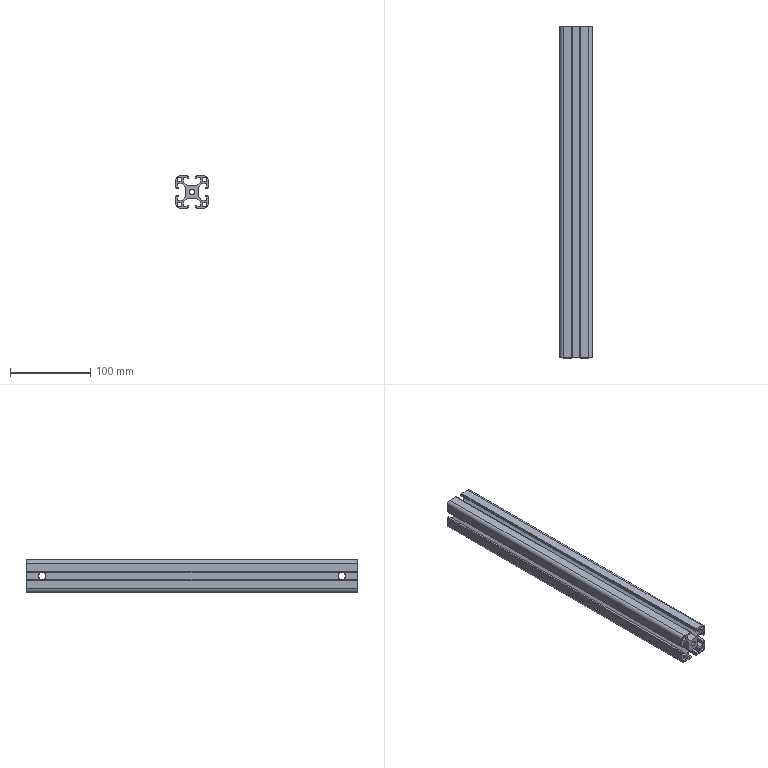Part | SolidWorks | features HoleWzd 1, WeldMemberFeat 1, WeldmentFeature 1 | 1 solid | 142 faces | box 40 x 413 x 40 mm | volume 248012 mm3 | plane 102 | cylinder 40 | commonest cylinder face diameters 9 x14 16 x12 6 x8 6.8 x6